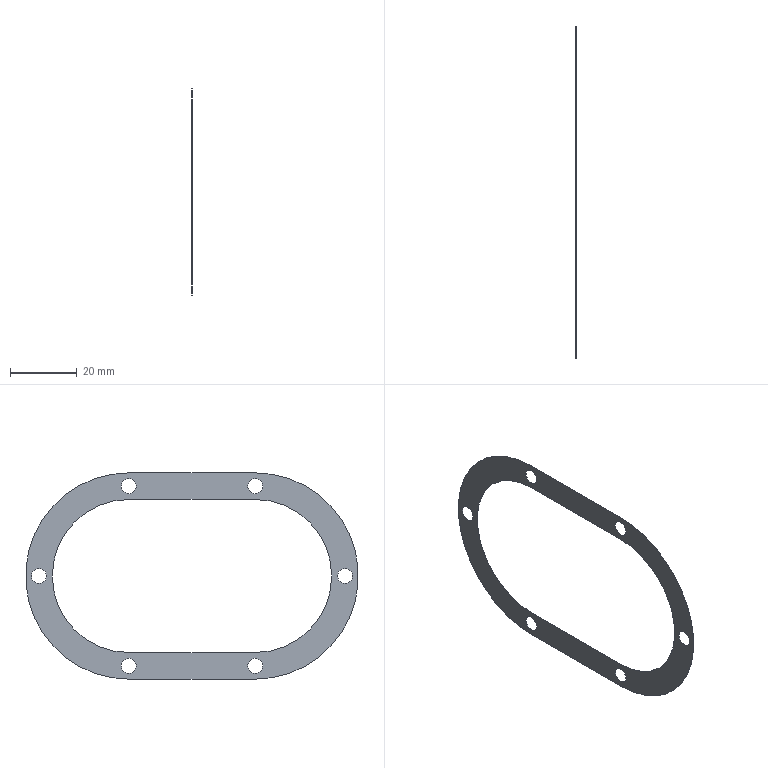Part | SolidWorks | features Extrusion 1 | 1 solid | 22 faces | box 0.05 x 100 x 62 mm | volume 93.487 mm3 | cylinder 16 | plane 6 | commonest cylinder face diameters 4.5 x12 46 x2 62 x2
STEP:
#1=CARTESIAN_POINT('',(0.,-46.,2.25));
#2=VERTEX_POINT('',#1);
#3=CARTESIAN_POINT('',(0.,-46.,-2.25));
#4=VERTEX_POINT('',#3);
#5=CARTESIAN_POINT('',(0.,-46.,0.));
#6=DIRECTION('',(1.,0.,0.));
#7=DIRECTION('',(0.,0.,1.));
#8=AXIS2_PLACEMENT_3D('',#5,#6,#7);
#9=CIRCLE('',#8,2.25);
#10=EDGE_CURVE('',#2,#4,#9,.T.);
#11=ORIENTED_EDGE('',*,*,#10,.F.);
#12=CARTESIAN_POINT('',(0.05,-46.,2.25));
#13=VERTEX_POINT('',#12);
#14=CARTESIAN_POINT('',(0.,-46.,2.25));
#15=DIRECTION('',(1.,0.,0.));
#16=VECTOR('',#15,1000.);
#17=LINE('',#14,#16);
#18=EDGE_CURVE('',#2,#13,#17,.T.);
#19=ORIENTED_EDGE('',*,*,#18,.T.);
#20=CARTESIAN_POINT('',(0.05,-46.,-2.25));
#21=VERTEX_POINT('',#20);
#22=CARTESIAN_POINT('',(0.05,-46.,0.));
#23=DIRECTION('',(1.,0.,0.));
#24=DIRECTION('',(0.,0.,1.));
#25=AXIS2_PLACEMENT_3D('',#22,#23,#24);
#26=CIRCLE('',#25,2.25);
#27=EDGE_CURVE('',#13,#21,#26,.T.);
#28=ORIENTED_EDGE('',*,*,#27,.T.);
#29=CARTESIAN_POINT('',(0.,-46.,-2.25));
#30=DIRECTION('',(1.,0.,0.));
#31=VECTOR('',#30,1000.);
#32=LINE('',#29,#31);
#33=EDGE_CURVE('',#4,#21,#32,.T.);
#34=ORIENTED_EDGE('',*,*,#33,.F.);
#35=EDGE_LOOP('',(#11,#19,#28,#34));
#36=FACE_OUTER_BOUND('',#35,.T.);
#37=CARTESIAN_POINT('',(0.,-46.,0.));
#38=DIRECTION('',(1.,0.,0.));
#39=DIRECTION('',(0.,0.,-1.));
#40=AXIS2_PLACEMENT_3D('',#37,#38,#39);
#41=CYLINDRICAL_SURFACE('',#40,2.25);
#42=ADVANCED_FACE('',(#36),#41,.F.);
#43=CARTESIAN_POINT('',(0.,-19.,29.25));
#44=VERTEX_POINT('',#43);
#45=CARTESIAN_POINT('',(0.,-19.,24.75));
#46=VERTEX_POINT('',#45);
#47=CARTESIAN_POINT('',(0.,-19.,27.));
#48=DIRECTION('',(1.,0.,0.));
#49=DIRECTION('',(0.,0.,1.));
#50=AXIS2_PLACEMENT_3D('',#47,#48,#49);
#51=CIRCLE('',#50,2.25);
#52=EDGE_CURVE('',#44,#46,#51,.T.);
#53=ORIENTED_EDGE('',*,*,#52,.F.);
#54=CARTESIAN_POINT('',(0.05,-19.,29.25));
#55=VERTEX_POINT('',#54);
#56=CARTESIAN_POINT('',(0.,-19.,29.25));
#57=DIRECTION('',(1.,0.,0.));
#58=VECTOR('',#57,1000.);
#59=LINE('',#56,#58);
#60=EDGE_CURVE('',#44,#55,#59,.T.);
#61=ORIENTED_EDGE('',*,*,#60,.T.);
#62=CARTESIAN_POINT('',(0.05,-19.,24.75));
#63=VERTEX_POINT('',#62);
#64=CARTESIAN_POINT('',(0.05,-19.,27.));
#65=DIRECTION('',(1.,0.,0.));
#66=DIRECTION('',(0.,0.,1.));
#67=AXIS2_PLACEMENT_3D('',#64,#65,#66);
#68=CIRCLE('',#67,2.25);
#69=EDGE_CURVE('',#55,#63,#68,.T.);
#70=ORIENTED_EDGE('',*,*,#69,.T.);
#71=CARTESIAN_POINT('',(0.,-19.,24.75));
#72=DIRECTION('',(1.,0.,0.));
#73=VECTOR('',#72,1000.);
#74=LINE('',#71,#73);
#75=EDGE_CURVE('',#46,#63,#74,.T.);
#76=ORIENTED_EDGE('',*,*,#75,.F.);
#77=EDGE_LOOP('',(#53,#61,#70,#76));
#78=FACE_OUTER_BOUND('',#77,.T.);
#79=CARTESIAN_POINT('',(0.,-19.,27.));
#80=DIRECTION('',(1.,0.,0.));
#81=DIRECTION('',(0.,0.,-1.));
#82=AXIS2_PLACEMENT_3D('',#79,#80,#81);
#83=CYLINDRICAL_SURFACE('',#82,2.25);
#84=ADVANCED_FACE('',(#78),#83,.F.);
#85=CARTESIAN_POINT('',(0.,19.,29.25));
#86=VERTEX_POINT('',#85);
#87=CARTESIAN_POINT('',(0.,19.,24.75));
#88=VERTEX_POINT('',#87);
#89=CARTESIAN_POINT('',(0.,19.,27.));
#90=DIRECTION('',(1.,0.,0.));
#91=DIRECTION('',(0.,0.,1.));
#92=AXIS2_PLACEMENT_3D('',#89,#90,#91);
#93=CIRCLE('',#92,2.25);
#94=EDGE_CURVE('',#86,#88,#93,.T.);
#95=ORIENTED_EDGE('',*,*,#94,.F.);
#96=CARTESIAN_POINT('',(0.05,19.,29.25));
#97=VERTEX_POINT('',#96);
#98=CARTESIAN_POINT('',(0.,19.,29.25));
#99=DIRECTION('',(1.,0.,0.));
#100=VECTOR('',#99,1000.);
#101=LINE('',#98,#100);
#102=EDGE_CURVE('',#86,#97,#101,.T.);
#103=ORIENTED_EDGE('',*,*,#102,.T.);
#104=CARTESIAN_POINT('',(0.05,19.,24.75));
#105=VERTEX_POINT('',#104);
#106=CARTESIAN_POINT('',(0.05,19.,27.));
#107=DIRECTION('',(1.,0.,0.));
#108=DIRECTION('',(0.,0.,1.));
#109=AXIS2_PLACEMENT_3D('',#106,#107,#108);
#110=CIRCLE('',#109,2.25);
#111=EDGE_CURVE('',#97,#105,#110,.T.);
#112=ORIENTED_EDGE('',*,*,#111,.T.);
#113=CARTESIAN_POINT('',(0.,19.,24.75));
#114=DIRECTION('',(1.,0.,0.));
#115=VECTOR('',#114,1000.);
#116=LINE('',#113,#115);
#117=EDGE_CURVE('',#88,#105,#116,.T.);
#118=ORIENTED_EDGE('',*,*,#117,.F.);
#119=EDGE_LOOP('',(#95,#103,#112,#118));
#120=FACE_OUTER_BOUND('',#119,.T.);
#121=CARTESIAN_POINT('',(0.,19.,27.));
#122=DIRECTION('',(1.,0.,0.));
#123=DIRECTION('',(0.,0.,-1.));
#124=AXIS2_PLACEMENT_3D('',#121,#122,#123);
#125=CYLINDRICAL_SURFACE('',#124,2.25);
#126=ADVANCED_FACE('',(#120),#125,.F.);
#127=CARTESIAN_POINT('',(0.,46.,2.25));
#128=VERTEX_POINT('',#127);
#129=CARTESIAN_POINT('',(0.,46.,-2.25));
#130=VERTEX_POINT('',#129);
#131=CARTESIAN_POINT('',(0.,46.,0.));
#132=DIRECTION('',(1.,0.,0.));
#133=DIRECTION('',(0.,0.,1.));
#134=AXIS2_PLACEMENT_3D('',#131,#132,#133);
#135=CIRCLE('',#134,2.25);
#136=EDGE_CURVE('',#128,#130,#135,.T.);
#137=ORIENTED_EDGE('',*,*,#136,.F.);
#138=CARTESIAN_POINT('',(0.05,46.,2.25));
#139=VERTEX_POINT('',#138);
#140=CARTESIAN_POINT('',(0.,46.,2.25));
#141=DIRECTION('',(1.,0.,0.));
#142=VECTOR('',#141,1000.);
#143=LINE('',#140,#142);
#144=EDGE_CURVE('',#128,#139,#143,.T.);
#145=ORIENTED_EDGE('',*,*,#144,.T.);
#146=CARTESIAN_POINT('',(0.05,46.,-2.25));
#147=VERTEX_POINT('',#146);
#148=CARTESIAN_POINT('',(0.05,46.,0.));
#149=DIRECTION('',(1.,0.,0.));
#150=DIRECTION('',(0.,0.,1.));
#151=AXIS2_PLACEMENT_3D('',#148,#149,#150);
#152=CIRCLE('',#151,2.25);
#153=EDGE_CURVE('',#139,#147,#152,.T.);
#154=ORIENTED_EDGE('',*,*,#153,.T.);
#155=CARTESIAN_POINT('',(0.,46.,-2.25));
#156=DIRECTION('',(1.,0.,0.));
#157=VECTOR('',#156,1000.);
#158=LINE('',#155,#157);
#159=EDGE_CURVE('',#130,#147,#158,.T.);
#160=ORIENTED_EDGE('',*,*,#159,.F.);
#161=EDGE_LOOP('',(#137,#145,#154,#160));
#162=FACE_OUTER_BOUND('',#161,.T.);
#163=CARTESIAN_POINT('',(0.,46.,0.));
#164=DIRECTION('',(1.,0.,0.));
#165=DIRECTION('',(0.,0.,-1.));
#166=AXIS2_PLACEMENT_3D('',#163,#164,#165);
#167=CYLINDRICAL_SURFACE('',#166,2.25);
#168=ADVANCED_FACE('',(#162),#167,.F.);
#169=CARTESIAN_POINT('',(0.,19.,-24.75));
#170=VERTEX_POINT('',#169);
#171=CARTESIAN_POINT('',(0.,19.,-29.25));
#172=VERTEX_POINT('',#171);
#173=CARTESIAN_POINT('',(0.,19.,-27.));
#174=DIRECTION('',(1.,0.,0.));
#175=DIRECTION('',(0.,0.,1.));
#176=AXIS2_PLACEMENT_3D('',#173,#174,#175);
#177=CIRCLE('',#176,2.25);
#178=EDGE_CURVE('',#170,#172,#177,.T.);
#179=ORIENTED_EDGE('',*,*,#178,.F.);
#180=CARTESIAN_POINT('',(0.05,19.,-24.75));
#181=VERTEX_POINT('',#180);
#182=CARTESIAN_POINT('',(0.,19.,-24.75));
#183=DIRECTION('',(1.,0.,0.));
#184=VECTOR('',#183,1000.);
#185=LINE('',#182,#184);
#186=EDGE_CURVE('',#170,#181,#185,.T.);
#187=ORIENTED_EDGE('',*,*,#186,.T.);
#188=CARTESIAN_POINT('',(0.05,19.,-29.25));
#189=VERTEX_POINT('',#188);
#190=CARTESIAN_POINT('',(0.05,19.,-27.));
#191=DIRECTION('',(1.,0.,0.));
#192=DIRECTION('',(0.,0.,1.));
#193=AXIS2_PLACEMENT_3D('',#190,#191,#192);
#194=CIRCLE('',#193,2.25);
#195=EDGE_CURVE('',#181,#189,#194,.T.);
#196=ORIENTED_EDGE('',*,*,#195,.T.);
#197=CARTESIAN_POINT('',(0.,19.,-29.25));
#198=DIRECTION('',(1.,0.,0.));
#199=VECTOR('',#198,1000.);
#200=LINE('',#197,#199);
#201=EDGE_CURVE('',#172,#189,#200,.T.);
#202=ORIENTED_EDGE('',*,*,#201,.F.);
#203=EDGE_LOOP('',(#179,#187,#196,#202));
#204=FACE_OUTER_BOUND('',#203,.T.);
#205=CARTESIAN_POINT('',(0.,19.,-27.));
#206=DIRECTION('',(1.,0.,0.));
#207=DIRECTION('',(0.,0.,-1.));
#208=AXIS2_PLACEMENT_3D('',#205,#206,#207);
#209=CYLINDRICAL_SURFACE('',#208,2.25);
#210=ADVANCED_FACE('',(#204),#209,.F.);
#211=CARTESIAN_POINT('',(0.,-19.,-24.75));
#212=VERTEX_POINT('',#211);
#213=CARTESIAN_POINT('',(0.,-19.,-29.25));
#214=VERTEX_POINT('',#213);
#215=CARTESIAN_POINT('',(0.,-19.,-27.));
#216=DIRECTION('',(1.,0.,0.));
#217=DIRECTION('',(0.,0.,1.));
#218=AXIS2_PLACEMENT_3D('',#215,#216,#217);
#219=CIRCLE('',#218,2.25);
#220=EDGE_CURVE('',#212,#214,#219,.T.);
#221=ORIENTED_EDGE('',*,*,#220,.F.);
#222=CARTESIAN_POINT('',(0.05,-19.,-24.75));
#223=VERTEX_POINT('',#222);
#224=CARTESIAN_POINT('',(0.,-19.,-24.75));
#225=DIRECTION('',(1.,0.,0.));
#226=VECTOR('',#225,1000.);
#227=LINE('',#224,#226);
#228=EDGE_CURVE('',#212,#223,#227,.T.);
#229=ORIENTED_EDGE('',*,*,#228,.T.);
#230=CARTESIAN_POINT('',(0.05,-19.,-29.25));
#231=VERTEX_POINT('',#230);
#232=CARTESIAN_POINT('',(0.05,-19.,-27.));
#233=DIRECTION('',(1.,0.,0.));
#234=DIRECTION('',(0.,0.,1.));
#235=AXIS2_PLACEMENT_3D('',#232,#233,#234);
#236=CIRCLE('',#235,2.25);
#237=EDGE_CURVE('',#223,#231,#236,.T.);
#238=ORIENTED_EDGE('',*,*,#237,.T.);
#239=CARTESIAN_POINT('',(0.,-19.,-29.25));
#240=DIRECTION('',(1.,0.,0.));
#241=VECTOR('',#240,1000.);
#242=LINE('',#239,#241);
#243=EDGE_CURVE('',#214,#231,#242,.T.);
#244=ORIENTED_EDGE('',*,*,#243,.F.);
#245=EDGE_LOOP('',(#221,#229,#238,#244));
#246=FACE_OUTER_BOUND('',#245,.T.);
#247=CARTESIAN_POINT('',(0.,-19.,-27.));
#248=DIRECTION('',(1.,0.,0.));
#249=DIRECTION('',(0.,0.,-1.));
#250=AXIS2_PLACEMENT_3D('',#247,#248,#249);
#251=CYLINDRICAL_SURFACE('',#250,2.25);
#252=ADVANCED_FACE('',(#246),#251,.F.);
#253=CARTESIAN_POINT('',(0.05,-19.,31.));
#254=VERTEX_POINT('',#253);
#255=CARTESIAN_POINT('',(0.05,-19.,-31.));
#256=VERTEX_POINT('',#255);
#257=CARTESIAN_POINT('',(0.05,-19.,0.));
#258=DIRECTION('',(1.,0.,0.));
#259=DIRECTION('',(0.,0.,-1.));
#260=AXIS2_PLACEMENT_3D('',#257,#258,#259);
#261=CIRCLE('',#260,31.);
#262=EDGE_CURVE('',#254,#256,#261,.T.);
#263=ORIENTED_EDGE('',*,*,#262,.F.);
#264=CARTESIAN_POINT('',(0.,-19.,31.));
#265=VERTEX_POINT('',#264);
#266=CARTESIAN_POINT('',(0.,-19.,31.));
#267=DIRECTION('',(1.,0.,0.));
#268=VECTOR('',#267,1000.);
#269=LINE('',#266,#268);
#270=EDGE_CURVE('',#265,#254,#269,.T.);
#271=ORIENTED_EDGE('',*,*,#270,.F.);
#272=CARTESIAN_POINT('',(0.,-19.,-31.));
#273=VERTEX_POINT('',#272);
#274=CARTESIAN_POINT('',(0.,-19.,0.));
#275=DIRECTION('',(1.,0.,0.));
#276=DIRECTION('',(0.,0.,-1.));
#277=AXIS2_PLACEMENT_3D('',#274,#275,#276);
#278=CIRCLE('',#277,31.);
#279=EDGE_CURVE('',#265,#273,#278,.T.);
#280=ORIENTED_EDGE('',*,*,#279,.T.);
#281=CARTESIAN_POINT('',(0.,-19.,-31.));
#282=DIRECTION('',(1.,0.,0.));
#283=VECTOR('',#282,1000.);
#284=LINE('',#281,#283);
#285=EDGE_CURVE('',#273,#256,#284,.T.);
#286=ORIENTED_EDGE('',*,*,#285,.T.);
#287=EDGE_LOOP('',(#263,#271,#280,#286));
#288=FACE_OUTER_BOUND('',#287,.T.);
#289=CARTESIAN_POINT('',(0.,-19.,0.));
#290=DIRECTION('',(1.,0.,0.));
#291=DIRECTION('',(0.,0.,-1.));
#292=AXIS2_PLACEMENT_3D('',#289,#290,#291);
#293=CYLINDRICAL_SURFACE('',#292,31.);
#294=ADVANCED_FACE('',(#288),#293,.T.);
#295=CARTESIAN_POINT('',(0.05,19.,31.));
#296=VERTEX_POINT('',#295);
#297=CARTESIAN_POINT('',(0.05,19.,31.));
#298=DIRECTION('',(0.,-1.,0.));
#299=VECTOR('',#298,1000.);
#300=LINE('',#297,#299);
#301=EDGE_CURVE('',#296,#254,#300,.T.);
#302=ORIENTED_EDGE('',*,*,#301,.F.);
#303=CARTESIAN_POINT('',(0.,19.,31.));
#304=VERTEX_POINT('',#303);
#305=CARTESIAN_POINT('',(0.,19.,31.));
#306=DIRECTION('',(1.,0.,0.));
#307=VECTOR('',#306,1000.);
#308=LINE('',#305,#307);
#309=EDGE_CURVE('',#304,#296,#308,.T.);
#310=ORIENTED_EDGE('',*,*,#309,.F.);
#311=CARTESIAN_POINT('',(0.,19.,31.));
#312=DIRECTION('',(0.,-1.,0.));
#313=VECTOR('',#312,1000.);
#314=LINE('',#311,#313);
#315=EDGE_CURVE('',#304,#265,#314,.T.);
#316=ORIENTED_EDGE('',*,*,#315,.T.);
#317=ORIENTED_EDGE('',*,*,#270,.T.);
#318=EDGE_LOOP('',(#302,#310,#316,#317));
#319=FACE_OUTER_BOUND('',#318,.T.);
#320=CARTESIAN_POINT('',(0.,19.,31.));
#321=DIRECTION('',(0.,0.,1.));
#322=DIRECTION('',(1.,0.,0.));
#323=AXIS2_PLACEMENT_3D('',#320,#321,#322);
#324=PLANE('',#323);
#325=ADVANCED_FACE('',(#319),#324,.T.);
#326=CARTESIAN_POINT('',(0.05,19.,-31.));
#327=VERTEX_POINT('',#326);
#328=CARTESIAN_POINT('',(0.05,19.,0.));
#329=DIRECTION('',(1.,0.,0.));
#330=DIRECTION('',(0.,0.,-1.));
#331=AXIS2_PLACEMENT_3D('',#328,#329,#330);
#332=CIRCLE('',#331,31.);
#333=EDGE_CURVE('',#327,#296,#332,.T.);
#334=ORIENTED_EDGE('',*,*,#333,.F.);
#335=CARTESIAN_POINT('',(0.,19.,-31.));
#336=VERTEX_POINT('',#335);
#337=CARTESIAN_POINT('',(0.,19.,-31.));
#338=DIRECTION('',(1.,0.,0.));
#339=VECTOR('',#338,1000.);
#340=LINE('',#337,#339);
#341=EDGE_CURVE('',#336,#327,#340,.T.);
#342=ORIENTED_EDGE('',*,*,#341,.F.);
#343=CARTESIAN_POINT('',(0.,19.,0.));
#344=DIRECTION('',(1.,0.,0.));
#345=DIRECTION('',(0.,0.,-1.));
#346=AXIS2_PLACEMENT_3D('',#343,#344,#345);
#347=CIRCLE('',#346,31.);
#348=EDGE_CURVE('',#336,#304,#347,.T.);
#349=ORIENTED_EDGE('',*,*,#348,.T.);
#350=ORIENTED_EDGE('',*,*,#309,.T.);
#351=EDGE_LOOP('',(#334,#342,#349,#350));
#352=FACE_OUTER_BOUND('',#351,.T.);
#353=CARTESIAN_POINT('',(0.,19.,0.));
#354=DIRECTION('',(1.,0.,0.));
#355=DIRECTION('',(0.,0.,-1.));
#356=AXIS2_PLACEMENT_3D('',#353,#354,#355);
#357=CYLINDRICAL_SURFACE('',#356,31.);
#358=ADVANCED_FACE('',(#352),#357,.T.);
#359=CARTESIAN_POINT('',(0.05,-19.,-31.));
#360=DIRECTION('',(0.,1.,0.));
#361=VECTOR('',#360,1000.);
#362=LINE('',#359,#361);
#363=EDGE_CURVE('',#256,#327,#362,.T.);
#364=ORIENTED_EDGE('',*,*,#363,.F.);
#365=ORIENTED_EDGE('',*,*,#285,.F.);
#366=CARTESIAN_POINT('',(0.,-19.,-31.));
#367=DIRECTION('',(0.,1.,0.));
#368=VECTOR('',#367,1000.);
#369=LINE('',#366,#368);
#370=EDGE_CURVE('',#273,#336,#369,.T.);
#371=ORIENTED_EDGE('',*,*,#370,.T.);
#372=ORIENTED_EDGE('',*,*,#341,.T.);
#373=EDGE_LOOP('',(#364,#365,#371,#372));
#374=FACE_OUTER_BOUND('',#373,.T.);
#375=CARTESIAN_POINT('',(0.,-19.,-31.));
#376=DIRECTION('',(0.,0.,-1.));
#377=DIRECTION('',(-1.,0.,0.));
#378=AXIS2_PLACEMENT_3D('',#375,#376,#377);
#379=PLANE('',#378);
#380=ADVANCED_FACE('',(#374),#379,.T.);
#381=CARTESIAN_POINT('',(0.,-46.,0.));
#382=DIRECTION('',(1.,0.,0.));
#383=DIRECTION('',(0.,0.,1.));
#384=AXIS2_PLACEMENT_3D('',#381,#382,#383);
#385=CIRCLE('',#384,2.25);
#386=EDGE_CURVE('',#4,#2,#385,.T.);
#387=ORIENTED_EDGE('',*,*,#386,.T.);
#388=ORIENTED_EDGE('',*,*,#10,.T.);
#389=EDGE_LOOP('',(#387,#388));
#390=FACE_BOUND('',#389,.T.);
#391=CARTESIAN_POINT('',(0.,-19.,27.));
#392=DIRECTION('',(1.,0.,0.));
#393=DIRECTION('',(0.,0.,1.));
#394=AXIS2_PLACEMENT_3D('',#391,#392,#393);
#395=CIRCLE('',#394,2.25);
#396=EDGE_CURVE('',#46,#44,#395,.T.);
#397=ORIENTED_EDGE('',*,*,#396,.T.);
#398=ORIENTED_EDGE('',*,*,#52,.T.);
#399=EDGE_LOOP('',(#397,#398));
#400=FACE_BOUND('',#399,.T.);
#401=CARTESIAN_POINT('',(0.,19.,27.));
#402=DIRECTION('',(1.,0.,0.));
#403=DIRECTION('',(0.,0.,1.));
#404=AXIS2_PLACEMENT_3D('',#401,#402,#403);
#405=CIRCLE('',#404,2.25);
#406=EDGE_CURVE('',#88,#86,#405,.T.);
#407=ORIENTED_EDGE('',*,*,#406,.T.);
#408=ORIENTED_EDGE('',*,*,#94,.T.);
#409=EDGE_LOOP('',(#407,#408));
#410=FACE_BOUND('',#409,.T.);
#411=CARTESIAN_POINT('',(0.,46.,0.));
#412=DIRECTION('',(1.,0.,0.));
#413=DIRECTION('',(0.,0.,1.));
#414=AXIS2_PLACEMENT_3D('',#411,#412,#413);
#415=CIRCLE('',#414,2.25);
#416=EDGE_CURVE('',#130,#128,#415,.T.);
#417=ORIENTED_EDGE('',*,*,#416,.T.);
#418=ORIENTED_EDGE('',*,*,#136,.T.);
#419=EDGE_LOOP('',(#417,#418));
#420=FACE_BOUND('',#419,.T.);
#421=CARTESIAN_POINT('',(0.,-19.,-23.));
#422=VERTEX_POINT('',#421);
#423=CARTESIAN_POINT('',(0.,19.,-23.));
#424=VERTEX_POINT('',#423);
#425=CARTESIAN_POINT('',(0.,19.,-23.));
#426=DIRECTION('',(0.,1.,0.));
#427=VECTOR('',#426,1000.);
#428=LINE('',#425,#427);
#429=EDGE_CURVE('',#422,#424,#428,.T.);
#430=ORIENTED_EDGE('',*,*,#429,.T.);
#431=CARTESIAN_POINT('',(0.,19.,23.));
#432=VERTEX_POINT('',#431);
#433=CARTESIAN_POINT('',(0.,19.,0.));
#434=DIRECTION('',(1.,0.,0.));
#435=DIRECTION('',(0.,0.,1.));
#436=AXIS2_PLACEMENT_3D('',#433,#434,#435);
#437=CIRCLE('',#436,23.);
#438=EDGE_CURVE('',#424,#432,#437,.T.);
#439=ORIENTED_EDGE('',*,*,#438,.T.);
#440=CARTESIAN_POINT('',(0.,-19.,23.));
#441=VERTEX_POINT('',#440);
#442=CARTESIAN_POINT('',(0.,-19.,23.));
#443=DIRECTION('',(0.,-1.,0.));
#444=VECTOR('',#443,1000.);
#445=LINE('',#442,#444);
#446=EDGE_CURVE('',#432,#441,#445,.T.);
#447=ORIENTED_EDGE('',*,*,#446,.T.);
#448=CARTESIAN_POINT('',(0.,-19.,0.));
#449=DIRECTION('',(1.,0.,0.));
#450=DIRECTION('',(0.,0.,1.));
#451=AXIS2_PLACEMENT_3D('',#448,#449,#450);
#452=CIRCLE('',#451,23.);
#453=EDGE_CURVE('',#441,#422,#452,.T.);
#454=ORIENTED_EDGE('',*,*,#453,.T.);
#455=EDGE_LOOP('',(#430,#439,#447,#454));
#456=FACE_BOUND('',#455,.T.);
#457=CARTESIAN_POINT('',(0.,19.,-27.));
#458=DIRECTION('',(1.,0.,0.));
#459=DIRECTION('',(0.,0.,1.));
#460=AXIS2_PLACEMENT_3D('',#457,#458,#459);
#461=CIRCLE('',#460,2.25);
#462=EDGE_CURVE('',#172,#170,#461,.T.);
#463=ORIENTED_EDGE('',*,*,#462,.T.);
#464=ORIENTED_EDGE('',*,*,#178,.T.);
#465=EDGE_LOOP('',(#463,#464));
#466=FACE_BOUND('',#465,.T.);
#467=CARTESIAN_POINT('',(0.,-19.,-27.));
#468=DIRECTION('',(1.,0.,0.));
#469=DIRECTION('',(0.,0.,1.));
#470=AXIS2_PLACEMENT_3D('',#467,#468,#469);
#471=CIRCLE('',#470,2.25);
#472=EDGE_CURVE('',#214,#212,#471,.T.);
#473=ORIENTED_EDGE('',*,*,#472,.T.);
#474=ORIENTED_EDGE('',*,*,#220,.T.);
#475=EDGE_LOOP('',(#473,#474));
#476=FACE_BOUND('',#475,.T.);
#477=ORIENTED_EDGE('',*,*,#279,.F.);
#478=ORIENTED_EDGE('',*,*,#315,.F.);
#479=ORIENTED_EDGE('',*,*,#348,.F.);
#480=ORIENTED_EDGE('',*,*,#370,.F.);
#481=EDGE_LOOP('',(#477,#478,#479,#480));
#482=FACE_OUTER_BOUND('',#481,.T.);
#483=CARTESIAN_POINT('',(0.,-19.,0.));
#484=DIRECTION('',(1.,0.,0.));
#485=DIRECTION('',(0.,0.,-1.));
#486=AXIS2_PLACEMENT_3D('',#483,#484,#485);
#487=PLANE('',#486);
#488=ADVANCED_FACE('',(#390,#400,#410,#420,#456,#466,#476,#482),#487,.F.);
#489=CARTESIAN_POINT('',(0.05,-46.,0.));
#490=DIRECTION('',(1.,0.,0.));
#491=DIRECTION('',(0.,0.,1.));
#492=AXIS2_PLACEMENT_3D('',#489,#490,#491);
#493=CIRCLE('',#492,2.25);
#494=EDGE_CURVE('',#21,#13,#493,.T.);
#495=ORIENTED_EDGE('',*,*,#494,.F.);
#496=ORIENTED_EDGE('',*,*,#27,.F.);
#497=EDGE_LOOP('',(#495,#496));
#498=FACE_BOUND('',#497,.T.);
#499=CARTESIAN_POINT('',(0.05,-19.,27.));
#500=DIRECTION('',(1.,0.,0.));
#501=DIRECTION('',(0.,0.,1.));
#502=AXIS2_PLACEMENT_3D('',#499,#500,#501);
#503=CIRCLE('',#502,2.25);
#504=EDGE_CURVE('',#63,#55,#503,.T.);
#505=ORIENTED_EDGE('',*,*,#504,.F.);
#506=ORIENTED_EDGE('',*,*,#69,.F.);
#507=EDGE_LOOP('',(#505,#506));
#508=FACE_BOUND('',#507,.T.);
#509=CARTESIAN_POINT('',(0.05,19.,27.));
#510=DIRECTION('',(1.,0.,0.));
#511=DIRECTION('',(0.,0.,1.));
#512=AXIS2_PLACEMENT_3D('',#509,#510,#511);
#513=CIRCLE('',#512,2.25);
#514=EDGE_CURVE('',#105,#97,#513,.T.);
#515=ORIENTED_EDGE('',*,*,#514,.F.);
#516=ORIENTED_EDGE('',*,*,#111,.F.);
#517=EDGE_LOOP('',(#515,#516));
#518=FACE_BOUND('',#517,.T.);
#519=CARTESIAN_POINT('',(0.05,46.,0.));
#520=DIRECTION('',(1.,0.,0.));
#521=DIRECTION('',(0.,0.,1.));
#522=AXIS2_PLACEMENT_3D('',#519,#520,#521);
#523=CIRCLE('',#522,2.25);
#524=EDGE_CURVE('',#147,#139,#523,.T.);
#525=ORIENTED_EDGE('',*,*,#524,.F.);
#526=ORIENTED_EDGE('',*,*,#153,.F.);
#527=EDGE_LOOP('',(#525,#526));
#528=FACE_BOUND('',#527,.T.);
#529=CARTESIAN_POINT('',(0.05,19.,-23.));
#530=VERTEX_POINT('',#529);
#531=CARTESIAN_POINT('',(0.05,19.,23.));
#532=VERTEX_POINT('',#531);
#533=CARTESIAN_POINT('',(0.05,19.,0.));
#534=DIRECTION('',(1.,0.,0.));
#535=DIRECTION('',(0.,0.,1.));
#536=AXIS2_PLACEMENT_3D('',#533,#534,#535);
#537=CIRCLE('',#536,23.);
#538=EDGE_CURVE('',#530,#532,#537,.T.);
#539=ORIENTED_EDGE('',*,*,#538,.F.);
#540=CARTESIAN_POINT('',(0.05,-19.,-23.));
#541=VERTEX_POINT('',#540);
#542=CARTESIAN_POINT('',(0.05,19.,-23.));
#543=DIRECTION('',(0.,1.,0.));
#544=VECTOR('',#543,1000.);
#545=LINE('',#542,#544);
#546=EDGE_CURVE('',#541,#530,#545,.T.);
#547=ORIENTED_EDGE('',*,*,#546,.F.);
#548=CARTESIAN_POINT('',(0.05,-19.,23.));
#549=VERTEX_POINT('',#548);
#550=CARTESIAN_POINT('',(0.05,-19.,0.));
#551=DIRECTION('',(1.,0.,0.));
#552=DIRECTION('',(0.,0.,1.));
#553=AXIS2_PLACEMENT_3D('',#550,#551,#552);
#554=CIRCLE('',#553,23.);
#555=EDGE_CURVE('',#549,#541,#554,.T.);
#556=ORIENTED_EDGE('',*,*,#555,.F.);
#557=CARTESIAN_POINT('',(0.05,-19.,23.));
#558=DIRECTION('',(0.,-1.,0.));
#559=VECTOR('',#558,1000.);
#560=LINE('',#557,#559);
#561=EDGE_CURVE('',#532,#549,#560,.T.);
#562=ORIENTED_EDGE('',*,*,#561,.F.);
#563=EDGE_LOOP('',(#539,#547,#556,#562));
#564=FACE_BOUND('',#563,.T.);
#565=CARTESIAN_POINT('',(0.05,19.,-27.));
#566=DIRECTION('',(1.,0.,0.));
#567=DIRECTION('',(0.,0.,1.));
#568=AXIS2_PLACEMENT_3D('',#565,#566,#567);
#569=CIRCLE('',#568,2.25);
#570=EDGE_CURVE('',#189,#181,#569,.T.);
#571=ORIENTED_EDGE('',*,*,#570,.F.);
#572=ORIENTED_EDGE('',*,*,#195,.F.);
#573=EDGE_LOOP('',(#571,#572));
#574=FACE_BOUND('',#573,.T.);
#575=CARTESIAN_POINT('',(0.05,-19.,-27.));
#576=DIRECTION('',(1.,0.,0.));
#577=DIRECTION('',(0.,0.,1.));
#578=AXIS2_PLACEMENT_3D('',#575,#576,#577);
#579=CIRCLE('',#578,2.25);
#580=EDGE_CURVE('',#231,#223,#579,.T.);
#581=ORIENTED_EDGE('',*,*,#580,.F.);
#582=ORIENTED_EDGE('',*,*,#237,.F.);
#583=EDGE_LOOP('',(#581,#582));
#584=FACE_BOUND('',#583,.T.);
#585=ORIENTED_EDGE('',*,*,#262,.T.);
#586=ORIENTED_EDGE('',*,*,#363,.T.);
#587=ORIENTED_EDGE('',*,*,#333,.T.);
#588=ORIENTED_EDGE('',*,*,#301,.T.);
#589=EDGE_LOOP('',(#585,#586,#587,#588));
#590=FACE_OUTER_BOUND('',#589,.T.);
#591=CARTESIAN_POINT('',(0.05,-19.,0.));
#592=DIRECTION('',(1.,0.,0.));
#593=DIRECTION('',(0.,0.,-1.));
#594=AXIS2_PLACEMENT_3D('',#591,#592,#593);
#595=PLANE('',#594);
#596=ADVANCED_FACE('',(#498,#508,#518,#528,#564,#574,#584,#590),#595,.T.);
#597=ORIENTED_EDGE('',*,*,#228,.F.);
#598=ORIENTED_EDGE('',*,*,#472,.F.);
#599=ORIENTED_EDGE('',*,*,#243,.T.);
#600=ORIENTED_EDGE('',*,*,#580,.T.);
#601=EDGE_LOOP('',(#597,#598,#599,#600));
#602=FACE_OUTER_BOUND('',#601,.T.);
#603=CARTESIAN_POINT('',(0.,-19.,-27.));
#604=DIRECTION('',(1.,0.,0.));
#605=DIRECTION('',(0.,0.,-1.));
#606=AXIS2_PLACEMENT_3D('',#603,#604,#605);
#607=CYLINDRICAL_SURFACE('',#606,2.25);
#608=ADVANCED_FACE('',(#602),#607,.F.);
#609=ORIENTED_EDGE('',*,*,#186,.F.);
#610=ORIENTED_EDGE('',*,*,#462,.F.);
#611=ORIENTED_EDGE('',*,*,#201,.T.);
#612=ORIENTED_EDGE('',*,*,#570,.T.);
#613=EDGE_LOOP('',(#609,#610,#611,#612));
#614=FACE_OUTER_BOUND('',#613,.T.);
#615=CARTESIAN_POINT('',(0.,19.,-27.));
#616=DIRECTION('',(1.,0.,0.));
#617=DIRECTION('',(0.,0.,-1.));
#618=AXIS2_PLACEMENT_3D('',#615,#616,#617);
#619=CYLINDRICAL_SURFACE('',#618,2.25);
#620=ADVANCED_FACE('',(#614),#619,.F.);
#621=ORIENTED_EDGE('',*,*,#538,.T.);
#622=CARTESIAN_POINT('',(0.,19.,23.));
#623=DIRECTION('',(1.,0.,0.));
#624=VECTOR('',#623,1000.);
#625=LINE('',#622,#624);
#626=EDGE_CURVE('',#432,#532,#625,.T.);
#627=ORIENTED_EDGE('',*,*,#626,.F.);
#628=ORIENTED_EDGE('',*,*,#438,.F.);
#629=CARTESIAN_POINT('',(0.,19.,-23.));
#630=DIRECTION('',(1.,0.,0.));
#631=VECTOR('',#630,1000.);
#632=LINE('',#629,#631);
#633=EDGE_CURVE('',#424,#530,#632,.T.);
#634=ORIENTED_EDGE('',*,*,#633,.T.);
#635=EDGE_LOOP('',(#621,#627,#628,#634));
#636=FACE_OUTER_BOUND('',#635,.T.);
#637=CARTESIAN_POINT('',(0.,19.,0.));
#638=DIRECTION('',(1.,0.,0.));
#639=DIRECTION('',(0.,0.,-1.));
#640=AXIS2_PLACEMENT_3D('',#637,#638,#639);
#641=CYLINDRICAL_SURFACE('',#640,23.);
#642=ADVANCED_FACE('',(#636),#641,.F.);
#643=ORIENTED_EDGE('',*,*,#546,.T.);
#644=ORIENTED_EDGE('',*,*,#633,.F.);
#645=ORIENTED_EDGE('',*,*,#429,.F.);
#646=CARTESIAN_POINT('',(0.,-19.,-23.));
#647=DIRECTION('',(1.,0.,0.));
#648=VECTOR('',#647,1000.);
#649=LINE('',#646,#648);
#650=EDGE_CURVE('',#422,#541,#649,.T.);
#651=ORIENTED_EDGE('',*,*,#650,.T.);
#652=EDGE_LOOP('',(#643,#644,#645,#651));
#653=FACE_OUTER_BOUND('',#652,.T.);
#654=CARTESIAN_POINT('',(0.,19.,-23.));
#655=DIRECTION('',(0.,0.,-1.));
#656=DIRECTION('',(-1.,0.,0.));
#657=AXIS2_PLACEMENT_3D('',#654,#655,#656);
#658=PLANE('',#657);
#659=ADVANCED_FACE('',(#653),#658,.F.);
#660=ORIENTED_EDGE('',*,*,#555,.T.);
#661=ORIENTED_EDGE('',*,*,#650,.F.);
#662=ORIENTED_EDGE('',*,*,#453,.F.);
#663=CARTESIAN_POINT('',(0.,-19.,23.));
#664=DIRECTION('',(1.,0.,0.));
#665=VECTOR('',#664,1000.);
#666=LINE('',#663,#665);
#667=EDGE_CURVE('',#441,#549,#666,.T.);
#668=ORIENTED_EDGE('',*,*,#667,.T.);
#669=EDGE_LOOP('',(#660,#661,#662,#668));
#670=FACE_OUTER_BOUND('',#669,.T.);
#671=CARTESIAN_POINT('',(0.,-19.,0.));
#672=DIRECTION('',(1.,0.,0.));
#673=DIRECTION('',(0.,0.,-1.));
#674=AXIS2_PLACEMENT_3D('',#671,#672,#673);
#675=CYLINDRICAL_SURFACE('',#674,23.);
#676=ADVANCED_FACE('',(#670),#675,.F.);
#677=ORIENTED_EDGE('',*,*,#561,.T.);
#678=ORIENTED_EDGE('',*,*,#667,.F.);
#679=ORIENTED_EDGE('',*,*,#446,.F.);
#680=ORIENTED_EDGE('',*,*,#626,.T.);
#681=EDGE_LOOP('',(#677,#678,#679,#680));
#682=FACE_OUTER_BOUND('',#681,.T.);
#683=CARTESIAN_POINT('',(0.,-19.,23.));
#684=DIRECTION('',(0.,0.,1.));
#685=DIRECTION('',(1.,0.,0.));
#686=AXIS2_PLACEMENT_3D('',#683,#684,#685);
#687=PLANE('',#686);
#688=ADVANCED_FACE('',(#682),#687,.F.);
#689=ORIENTED_EDGE('',*,*,#144,.F.);
#690=ORIENTED_EDGE('',*,*,#416,.F.);
#691=ORIENTED_EDGE('',*,*,#159,.T.);
#692=ORIENTED_EDGE('',*,*,#524,.T.);
#693=EDGE_LOOP('',(#689,#690,#691,#692));
#694=FACE_OUTER_BOUND('',#693,.T.);
#695=CARTESIAN_POINT('',(0.,46.,0.));
#696=DIRECTION('',(1.,0.,0.));
#697=DIRECTION('',(0.,0.,-1.));
#698=AXIS2_PLACEMENT_3D('',#695,#696,#697);
#699=CYLINDRICAL_SURFACE('',#698,2.25);
#700=ADVANCED_FACE('',(#694),#699,.F.);
#701=ORIENTED_EDGE('',*,*,#102,.F.);
#702=ORIENTED_EDGE('',*,*,#406,.F.);
#703=ORIENTED_EDGE('',*,*,#117,.T.);
#704=ORIENTED_EDGE('',*,*,#514,.T.);
#705=EDGE_LOOP('',(#701,#702,#703,#704));
#706=FACE_OUTER_BOUND('',#705,.T.);
#707=CARTESIAN_POINT('',(0.,19.,27.));
#708=DIRECTION('',(1.,0.,0.));
#709=DIRECTION('',(0.,0.,-1.));
#710=AXIS2_PLACEMENT_3D('',#707,#708,#709);
#711=CYLINDRICAL_SURFACE('',#710,2.25);
#712=ADVANCED_FACE('',(#706),#711,.F.);
#713=ORIENTED_EDGE('',*,*,#60,.F.);
#714=ORIENTED_EDGE('',*,*,#396,.F.);
#715=ORIENTED_EDGE('',*,*,#75,.T.);
#716=ORIENTED_EDGE('',*,*,#504,.T.);
#717=EDGE_LOOP('',(#713,#714,#715,#716));
#718=FACE_OUTER_BOUND('',#717,.T.);
#719=CARTESIAN_POINT('',(0.,-19.,27.));
#720=DIRECTION('',(1.,0.,0.));
#721=DIRECTION('',(0.,0.,-1.));
#722=AXIS2_PLACEMENT_3D('',#719,#720,#721);
#723=CYLINDRICAL_SURFACE('',#722,2.25);
#724=ADVANCED_FACE('',(#718),#723,.F.);
#725=ORIENTED_EDGE('',*,*,#18,.F.);
#726=ORIENTED_EDGE('',*,*,#386,.F.);
#727=ORIENTED_EDGE('',*,*,#33,.T.);
#728=ORIENTED_EDGE('',*,*,#494,.T.);
#729=EDGE_LOOP('',(#725,#726,#727,#728));
#730=FACE_OUTER_BOUND('',#729,.T.);
#731=CARTESIAN_POINT('',(0.,-46.,0.));
#732=DIRECTION('',(1.,0.,0.));
#733=DIRECTION('',(0.,0.,-1.));
#734=AXIS2_PLACEMENT_3D('',#731,#732,#733);
#735=CYLINDRICAL_SURFACE('',#734,2.25);
#736=ADVANCED_FACE('',(#730),#735,.F.);
#737=CLOSED_SHELL('',(#42,#84,#126,#168,#210,#252,#294,#325,#358,#380,#488,#596,#608,#620,#642,#659,#676,#688,#700,#712,#724,#736));
#738=MANIFOLD_SOLID_BREP('',#737);
#739=CARTESIAN_POINT('',(0.,0.,0.));
#740=DIRECTION('',(0.,0.,1.));
#741=DIRECTION('',(1.,0.,0.));
#742=AXIS2_PLACEMENT_3D('',#739,#740,#741);
#743=(LENGTH_UNIT()NAMED_UNIT(*)SI_UNIT(.MILLI.,.METRE.));
#744=UNCERTAINTY_MEASURE_WITH_UNIT(LENGTH_MEASURE(0.00001),#743,'','');
#745=(NAMED_UNIT(*)PLANE_ANGLE_UNIT()SI_UNIT($,.RADIAN.));
#746=(NAMED_UNIT(*)SI_UNIT($,.STERADIAN.)SOLID_ANGLE_UNIT());
#747=(GEOMETRIC_REPRESENTATION_CONTEXT(3)GLOBAL_UNCERTAINTY_ASSIGNED_CONTEXT((#744))GLOBAL_UNIT_ASSIGNED_CONTEXT((#743,#745,#746))REPRESENTATION_CONTEXT('',''));
#748=ADVANCED_BREP_SHAPE_REPRESENTATION('',(#738,#742),#747);